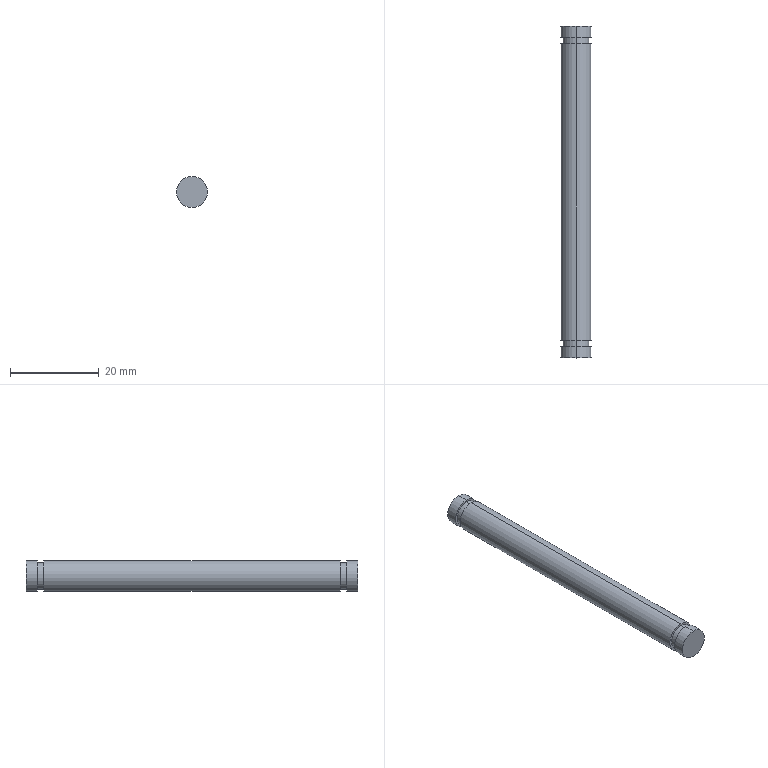Part | SolidWorks | features BaseBody 1 | 1 solid | 16 faces | box 7 x 75 x 7 mm | volume 2856 mm3 | cylinder 10 | plane 6 | commonest cylinder face diameters 7 x6 6 x4
STEP:
#1=CARTESIAN_POINT('',(896.946,-3867.373,951.471));
#2=VERTEX_POINT('',#1);
#3=CARTESIAN_POINT('',(896.946,-3867.373,958.471));
#4=VERTEX_POINT('',#3);
#5=CARTESIAN_POINT('',(896.946,-3867.373,954.971));
#6=DIRECTION('',(0.,-1.,0.));
#7=DIRECTION('',(0.,0.,-1.));
#8=AXIS2_PLACEMENT_3D('',#5,#6,#7);
#9=CIRCLE('',#8,3.5);
#10=EDGE_CURVE('',#2,#4,#9,.T.);
#11=ORIENTED_EDGE('',*,*,#10,.T.);
#12=CARTESIAN_POINT('',(896.946,-3934.373,958.471));
#13=VERTEX_POINT('',#12);
#14=CARTESIAN_POINT('',(896.946,-3903.373,958.471));
#15=DIRECTION('',(0.,-1.,0.));
#16=VECTOR('',#15,1000.);
#17=LINE('',#14,#16);
#18=EDGE_CURVE('',#4,#13,#17,.T.);
#19=ORIENTED_EDGE('',*,*,#18,.T.);
#20=CARTESIAN_POINT('',(896.946,-3934.373,951.471));
#21=VERTEX_POINT('',#20);
#22=CARTESIAN_POINT('',(896.946,-3934.373,954.971));
#23=DIRECTION('',(0.,1.,0.));
#24=DIRECTION('',(0.,0.,-1.));
#25=AXIS2_PLACEMENT_3D('',#22,#23,#24);
#26=CIRCLE('',#25,3.5);
#27=EDGE_CURVE('',#13,#21,#26,.T.);
#28=ORIENTED_EDGE('',*,*,#27,.T.);
#29=CARTESIAN_POINT('',(896.946,-3903.373,951.471));
#30=DIRECTION('',(0.,-1.,0.));
#31=VECTOR('',#30,1000.);
#32=LINE('',#29,#31);
#33=EDGE_CURVE('',#2,#21,#32,.T.);
#34=ORIENTED_EDGE('',*,*,#33,.F.);
#35=EDGE_LOOP('',(#11,#19,#28,#34));
#36=FACE_OUTER_BOUND('',#35,.T.);
#37=CARTESIAN_POINT('',(896.946,-3903.373,954.971));
#38=DIRECTION('',(0.,-1.,0.));
#39=DIRECTION('',(0.,0.,-1.));
#40=AXIS2_PLACEMENT_3D('',#37,#38,#39);
#41=CYLINDRICAL_SURFACE('',#40,3.5);
#42=ADVANCED_FACE('',(#36),#41,.T.);
#43=CARTESIAN_POINT('',(896.946,-3934.373,951.971));
#44=VERTEX_POINT('',#43);
#45=CARTESIAN_POINT('',(896.946,-3934.373,957.971));
#46=VERTEX_POINT('',#45);
#47=CARTESIAN_POINT('',(896.946,-3934.373,954.971));
#48=DIRECTION('',(0.,-1.,0.));
#49=DIRECTION('',(0.,0.,-1.));
#50=AXIS2_PLACEMENT_3D('',#47,#48,#49);
#51=CIRCLE('',#50,3.);
#52=EDGE_CURVE('',#44,#46,#51,.T.);
#53=ORIENTED_EDGE('',*,*,#52,.T.);
#54=CARTESIAN_POINT('',(896.946,-3935.873,957.971));
#55=VERTEX_POINT('',#54);
#56=CARTESIAN_POINT('',(896.946,-3938.667,957.971));
#57=DIRECTION('',(0.,-1.,0.));
#58=VECTOR('',#57,1000.);
#59=LINE('',#56,#58);
#60=EDGE_CURVE('',#46,#55,#59,.T.);
#61=ORIENTED_EDGE('',*,*,#60,.T.);
#62=CARTESIAN_POINT('',(896.946,-3935.873,951.971));
#63=VERTEX_POINT('',#62);
#64=CARTESIAN_POINT('',(896.946,-3935.873,954.971));
#65=DIRECTION('',(0.,1.,0.));
#66=DIRECTION('',(0.,0.,-1.));
#67=AXIS2_PLACEMENT_3D('',#64,#65,#66);
#68=CIRCLE('',#67,3.);
#69=EDGE_CURVE('',#55,#63,#68,.T.);
#70=ORIENTED_EDGE('',*,*,#69,.T.);
#71=CARTESIAN_POINT('',(896.946,-3938.667,951.971));
#72=DIRECTION('',(0.,-1.,0.));
#73=VECTOR('',#72,1000.);
#74=LINE('',#71,#73);
#75=EDGE_CURVE('',#44,#63,#74,.T.);
#76=ORIENTED_EDGE('',*,*,#75,.F.);
#77=EDGE_LOOP('',(#53,#61,#70,#76));
#78=FACE_OUTER_BOUND('',#77,.T.);
#79=CARTESIAN_POINT('',(896.946,-3938.667,954.971));
#80=DIRECTION('',(0.,-1.,0.));
#81=DIRECTION('',(0.,0.,-1.));
#82=AXIS2_PLACEMENT_3D('',#79,#80,#81);
#83=CYLINDRICAL_SURFACE('',#82,3.);
#84=ADVANCED_FACE('',(#78),#83,.T.);
#85=CARTESIAN_POINT('',(896.946,-3865.873,951.971));
#86=VERTEX_POINT('',#85);
#87=CARTESIAN_POINT('',(896.946,-3865.873,957.971));
#88=VERTEX_POINT('',#87);
#89=CARTESIAN_POINT('',(896.946,-3865.873,954.971));
#90=DIRECTION('',(0.,-1.,0.));
#91=DIRECTION('',(0.,0.,-1.));
#92=AXIS2_PLACEMENT_3D('',#89,#90,#91);
#93=CIRCLE('',#92,3.);
#94=EDGE_CURVE('',#86,#88,#93,.T.);
#95=ORIENTED_EDGE('',*,*,#94,.T.);
#96=CARTESIAN_POINT('',(896.946,-3867.373,957.971));
#97=VERTEX_POINT('',#96);
#98=CARTESIAN_POINT('',(896.946,-3870.167,957.971));
#99=DIRECTION('',(0.,-1.,0.));
#100=VECTOR('',#99,1000.);
#101=LINE('',#98,#100);
#102=EDGE_CURVE('',#88,#97,#101,.T.);
#103=ORIENTED_EDGE('',*,*,#102,.T.);
#104=CARTESIAN_POINT('',(896.946,-3867.373,951.971));
#105=VERTEX_POINT('',#104);
#106=CARTESIAN_POINT('',(896.946,-3867.373,954.971));
#107=DIRECTION('',(0.,1.,0.));
#108=DIRECTION('',(0.,0.,-1.));
#109=AXIS2_PLACEMENT_3D('',#106,#107,#108);
#110=CIRCLE('',#109,3.);
#111=EDGE_CURVE('',#97,#105,#110,.T.);
#112=ORIENTED_EDGE('',*,*,#111,.T.);
#113=CARTESIAN_POINT('',(896.946,-3870.167,951.971));
#114=DIRECTION('',(0.,-1.,0.));
#115=VECTOR('',#114,1000.);
#116=LINE('',#113,#115);
#117=EDGE_CURVE('',#86,#105,#116,.T.);
#118=ORIENTED_EDGE('',*,*,#117,.F.);
#119=EDGE_LOOP('',(#95,#103,#112,#118));
#120=FACE_OUTER_BOUND('',#119,.T.);
#121=CARTESIAN_POINT('',(896.946,-3870.167,954.971));
#122=DIRECTION('',(0.,-1.,0.));
#123=DIRECTION('',(0.,0.,-1.));
#124=AXIS2_PLACEMENT_3D('',#121,#122,#123);
#125=CYLINDRICAL_SURFACE('',#124,3.);
#126=ADVANCED_FACE('',(#120),#125,.T.);
#127=CARTESIAN_POINT('',(896.946,-3935.873,951.471));
#128=VERTEX_POINT('',#127);
#129=CARTESIAN_POINT('',(896.946,-3935.873,958.471));
#130=VERTEX_POINT('',#129);
#131=CARTESIAN_POINT('',(896.946,-3935.873,954.971));
#132=DIRECTION('',(0.,-1.,0.));
#133=DIRECTION('',(0.,0.,-1.));
#134=AXIS2_PLACEMENT_3D('',#131,#132,#133);
#135=CIRCLE('',#134,3.5);
#136=EDGE_CURVE('',#128,#130,#135,.T.);
#137=ORIENTED_EDGE('',*,*,#136,.T.);
#138=CARTESIAN_POINT('',(896.946,-3938.373,958.471));
#139=VERTEX_POINT('',#138);
#140=CARTESIAN_POINT('',(896.946,-3903.373,958.471));
#141=DIRECTION('',(0.,-1.,0.));
#142=VECTOR('',#141,1000.);
#143=LINE('',#140,#142);
#144=EDGE_CURVE('',#130,#139,#143,.T.);
#145=ORIENTED_EDGE('',*,*,#144,.T.);
#146=CARTESIAN_POINT('',(896.946,-3938.373,951.471));
#147=VERTEX_POINT('',#146);
#148=CARTESIAN_POINT('',(896.946,-3938.373,954.971));
#149=DIRECTION('',(0.,1.,0.));
#150=DIRECTION('',(0.,0.,-1.));
#151=AXIS2_PLACEMENT_3D('',#148,#149,#150);
#152=CIRCLE('',#151,3.5);
#153=EDGE_CURVE('',#139,#147,#152,.T.);
#154=ORIENTED_EDGE('',*,*,#153,.T.);
#155=CARTESIAN_POINT('',(896.946,-3903.373,951.471));
#156=DIRECTION('',(0.,-1.,0.));
#157=VECTOR('',#156,1000.);
#158=LINE('',#155,#157);
#159=EDGE_CURVE('',#128,#147,#158,.T.);
#160=ORIENTED_EDGE('',*,*,#159,.F.);
#161=EDGE_LOOP('',(#137,#145,#154,#160));
#162=FACE_OUTER_BOUND('',#161,.T.);
#163=CARTESIAN_POINT('',(896.946,-3903.373,954.971));
#164=DIRECTION('',(0.,-1.,0.));
#165=DIRECTION('',(0.,0.,-1.));
#166=AXIS2_PLACEMENT_3D('',#163,#164,#165);
#167=CYLINDRICAL_SURFACE('',#166,3.5);
#168=ADVANCED_FACE('',(#162),#167,.T.);
#169=CARTESIAN_POINT('',(896.946,-3863.373,951.471));
#170=VERTEX_POINT('',#169);
#171=CARTESIAN_POINT('',(896.946,-3863.373,958.471));
#172=VERTEX_POINT('',#171);
#173=CARTESIAN_POINT('',(896.946,-3863.373,954.971));
#174=DIRECTION('',(0.,-1.,0.));
#175=DIRECTION('',(0.,0.,-1.));
#176=AXIS2_PLACEMENT_3D('',#173,#174,#175);
#177=CIRCLE('',#176,3.5);
#178=EDGE_CURVE('',#170,#172,#177,.T.);
#179=ORIENTED_EDGE('',*,*,#178,.T.);
#180=CARTESIAN_POINT('',(896.946,-3865.873,958.471));
#181=VERTEX_POINT('',#180);
#182=CARTESIAN_POINT('',(896.946,-3903.373,958.471));
#183=DIRECTION('',(0.,-1.,0.));
#184=VECTOR('',#183,1000.);
#185=LINE('',#182,#184);
#186=EDGE_CURVE('',#172,#181,#185,.T.);
#187=ORIENTED_EDGE('',*,*,#186,.T.);
#188=CARTESIAN_POINT('',(896.946,-3865.873,951.471));
#189=VERTEX_POINT('',#188);
#190=CARTESIAN_POINT('',(896.946,-3865.873,954.971));
#191=DIRECTION('',(0.,1.,0.));
#192=DIRECTION('',(0.,0.,-1.));
#193=AXIS2_PLACEMENT_3D('',#190,#191,#192);
#194=CIRCLE('',#193,3.5);
#195=EDGE_CURVE('',#181,#189,#194,.T.);
#196=ORIENTED_EDGE('',*,*,#195,.T.);
#197=CARTESIAN_POINT('',(896.946,-3903.373,951.471));
#198=DIRECTION('',(0.,-1.,0.));
#199=VECTOR('',#198,1000.);
#200=LINE('',#197,#199);
#201=EDGE_CURVE('',#170,#189,#200,.T.);
#202=ORIENTED_EDGE('',*,*,#201,.F.);
#203=EDGE_LOOP('',(#179,#187,#196,#202));
#204=FACE_OUTER_BOUND('',#203,.T.);
#205=CARTESIAN_POINT('',(896.946,-3903.373,954.971));
#206=DIRECTION('',(0.,-1.,0.));
#207=DIRECTION('',(0.,0.,-1.));
#208=AXIS2_PLACEMENT_3D('',#205,#206,#207);
#209=CYLINDRICAL_SURFACE('',#208,3.5);
#210=ADVANCED_FACE('',(#204),#209,.T.);
#211=ORIENTED_EDGE('',*,*,#18,.F.);
#212=CARTESIAN_POINT('',(896.946,-3867.373,954.971));
#213=DIRECTION('',(0.,-1.,0.));
#214=DIRECTION('',(0.,0.,-1.));
#215=AXIS2_PLACEMENT_3D('',#212,#213,#214);
#216=CIRCLE('',#215,3.5);
#217=EDGE_CURVE('',#4,#2,#216,.T.);
#218=ORIENTED_EDGE('',*,*,#217,.T.);
#219=ORIENTED_EDGE('',*,*,#33,.T.);
#220=CARTESIAN_POINT('',(896.946,-3934.373,954.971));
#221=DIRECTION('',(0.,1.,0.));
#222=DIRECTION('',(0.,0.,-1.));
#223=AXIS2_PLACEMENT_3D('',#220,#221,#222);
#224=CIRCLE('',#223,3.5);
#225=EDGE_CURVE('',#21,#13,#224,.T.);
#226=ORIENTED_EDGE('',*,*,#225,.T.);
#227=EDGE_LOOP('',(#211,#218,#219,#226));
#228=FACE_OUTER_BOUND('',#227,.T.);
#229=CARTESIAN_POINT('',(896.946,-3903.373,954.971));
#230=DIRECTION('',(0.,-1.,0.));
#231=DIRECTION('',(0.,0.,-1.));
#232=AXIS2_PLACEMENT_3D('',#229,#230,#231);
#233=CYLINDRICAL_SURFACE('',#232,3.5);
#234=ADVANCED_FACE('',(#228),#233,.T.);
#235=ORIENTED_EDGE('',*,*,#52,.F.);
#236=CARTESIAN_POINT('',(896.946,-3934.373,954.971));
#237=DIRECTION('',(0.,-1.,0.));
#238=DIRECTION('',(0.,0.,-1.));
#239=AXIS2_PLACEMENT_3D('',#236,#237,#238);
#240=CIRCLE('',#239,3.);
#241=EDGE_CURVE('',#46,#44,#240,.T.);
#242=ORIENTED_EDGE('',*,*,#241,.F.);
#243=EDGE_LOOP('',(#235,#242));
#244=FACE_BOUND('',#243,.T.);
#245=ORIENTED_EDGE('',*,*,#225,.F.);
#246=ORIENTED_EDGE('',*,*,#27,.F.);
#247=EDGE_LOOP('',(#245,#246));
#248=FACE_OUTER_BOUND('',#247,.T.);
#249=CARTESIAN_POINT('',(896.946,-3934.373,954.971));
#250=DIRECTION('',(0.,1.,0.));
#251=DIRECTION('',(0.,0.,1.));
#252=AXIS2_PLACEMENT_3D('',#249,#250,#251);
#253=PLANE('',#252);
#254=ADVANCED_FACE('',(#244,#248),#253,.F.);
#255=CARTESIAN_POINT('',(896.946,-3867.373,954.971));
#256=DIRECTION('',(0.,1.,0.));
#257=DIRECTION('',(0.,0.,-1.));
#258=AXIS2_PLACEMENT_3D('',#255,#256,#257);
#259=CIRCLE('',#258,3.);
#260=EDGE_CURVE('',#105,#97,#259,.T.);
#261=ORIENTED_EDGE('',*,*,#260,.F.);
#262=ORIENTED_EDGE('',*,*,#111,.F.);
#263=EDGE_LOOP('',(#261,#262));
#264=FACE_BOUND('',#263,.T.);
#265=ORIENTED_EDGE('',*,*,#10,.F.);
#266=ORIENTED_EDGE('',*,*,#217,.F.);
#267=EDGE_LOOP('',(#265,#266));
#268=FACE_OUTER_BOUND('',#267,.T.);
#269=CARTESIAN_POINT('',(896.946,-3867.373,954.971));
#270=DIRECTION('',(0.,-1.,0.));
#271=DIRECTION('',(0.,0.,-1.));
#272=AXIS2_PLACEMENT_3D('',#269,#270,#271);
#273=PLANE('',#272);
#274=ADVANCED_FACE('',(#264,#268),#273,.F.);
#275=ORIENTED_EDGE('',*,*,#60,.F.);
#276=ORIENTED_EDGE('',*,*,#241,.T.);
#277=ORIENTED_EDGE('',*,*,#75,.T.);
#278=CARTESIAN_POINT('',(896.946,-3935.873,954.971));
#279=DIRECTION('',(0.,1.,0.));
#280=DIRECTION('',(0.,0.,-1.));
#281=AXIS2_PLACEMENT_3D('',#278,#279,#280);
#282=CIRCLE('',#281,3.);
#283=EDGE_CURVE('',#63,#55,#282,.T.);
#284=ORIENTED_EDGE('',*,*,#283,.T.);
#285=EDGE_LOOP('',(#275,#276,#277,#284));
#286=FACE_OUTER_BOUND('',#285,.T.);
#287=CARTESIAN_POINT('',(896.946,-3938.667,954.971));
#288=DIRECTION('',(0.,-1.,0.));
#289=DIRECTION('',(0.,0.,-1.));
#290=AXIS2_PLACEMENT_3D('',#287,#288,#289);
#291=CYLINDRICAL_SURFACE('',#290,3.);
#292=ADVANCED_FACE('',(#286),#291,.T.);
#293=ORIENTED_EDGE('',*,*,#102,.F.);
#294=CARTESIAN_POINT('',(896.946,-3865.873,954.971));
#295=DIRECTION('',(0.,-1.,0.));
#296=DIRECTION('',(0.,0.,-1.));
#297=AXIS2_PLACEMENT_3D('',#294,#295,#296);
#298=CIRCLE('',#297,3.);
#299=EDGE_CURVE('',#88,#86,#298,.T.);
#300=ORIENTED_EDGE('',*,*,#299,.T.);
#301=ORIENTED_EDGE('',*,*,#117,.T.);
#302=ORIENTED_EDGE('',*,*,#260,.T.);
#303=EDGE_LOOP('',(#293,#300,#301,#302));
#304=FACE_OUTER_BOUND('',#303,.T.);
#305=CARTESIAN_POINT('',(896.946,-3870.167,954.971));
#306=DIRECTION('',(0.,-1.,0.));
#307=DIRECTION('',(0.,0.,-1.));
#308=AXIS2_PLACEMENT_3D('',#305,#306,#307);
#309=CYLINDRICAL_SURFACE('',#308,3.);
#310=ADVANCED_FACE('',(#304),#309,.T.);
#311=ORIENTED_EDGE('',*,*,#283,.F.);
#312=ORIENTED_EDGE('',*,*,#69,.F.);
#313=EDGE_LOOP('',(#311,#312));
#314=FACE_BOUND('',#313,.T.);
#315=ORIENTED_EDGE('',*,*,#136,.F.);
#316=CARTESIAN_POINT('',(896.946,-3935.873,954.971));
#317=DIRECTION('',(0.,-1.,0.));
#318=DIRECTION('',(0.,0.,-1.));
#319=AXIS2_PLACEMENT_3D('',#316,#317,#318);
#320=CIRCLE('',#319,3.5);
#321=EDGE_CURVE('',#130,#128,#320,.T.);
#322=ORIENTED_EDGE('',*,*,#321,.F.);
#323=EDGE_LOOP('',(#315,#322));
#324=FACE_OUTER_BOUND('',#323,.T.);
#325=CARTESIAN_POINT('',(896.946,-3935.873,954.971));
#326=DIRECTION('',(0.,-1.,0.));
#327=DIRECTION('',(0.,0.,-1.));
#328=AXIS2_PLACEMENT_3D('',#325,#326,#327);
#329=PLANE('',#328);
#330=ADVANCED_FACE('',(#314,#324),#329,.F.);
#331=ORIENTED_EDGE('',*,*,#94,.F.);
#332=ORIENTED_EDGE('',*,*,#299,.F.);
#333=EDGE_LOOP('',(#331,#332));
#334=FACE_BOUND('',#333,.T.);
#335=CARTESIAN_POINT('',(896.946,-3865.873,954.971));
#336=DIRECTION('',(0.,1.,0.));
#337=DIRECTION('',(0.,0.,-1.));
#338=AXIS2_PLACEMENT_3D('',#335,#336,#337);
#339=CIRCLE('',#338,3.5);
#340=EDGE_CURVE('',#189,#181,#339,.T.);
#341=ORIENTED_EDGE('',*,*,#340,.F.);
#342=ORIENTED_EDGE('',*,*,#195,.F.);
#343=EDGE_LOOP('',(#341,#342));
#344=FACE_OUTER_BOUND('',#343,.T.);
#345=CARTESIAN_POINT('',(896.946,-3865.873,954.971));
#346=DIRECTION('',(0.,1.,0.));
#347=DIRECTION('',(0.,0.,1.));
#348=AXIS2_PLACEMENT_3D('',#345,#346,#347);
#349=PLANE('',#348);
#350=ADVANCED_FACE('',(#334,#344),#349,.F.);
#351=ORIENTED_EDGE('',*,*,#144,.F.);
#352=ORIENTED_EDGE('',*,*,#321,.T.);
#353=ORIENTED_EDGE('',*,*,#159,.T.);
#354=CARTESIAN_POINT('',(896.946,-3938.373,954.971));
#355=DIRECTION('',(0.,1.,0.));
#356=DIRECTION('',(0.,0.,-1.));
#357=AXIS2_PLACEMENT_3D('',#354,#355,#356);
#358=CIRCLE('',#357,3.5);
#359=EDGE_CURVE('',#147,#139,#358,.T.);
#360=ORIENTED_EDGE('',*,*,#359,.T.);
#361=EDGE_LOOP('',(#351,#352,#353,#360));
#362=FACE_OUTER_BOUND('',#361,.T.);
#363=CARTESIAN_POINT('',(896.946,-3903.373,954.971));
#364=DIRECTION('',(0.,-1.,0.));
#365=DIRECTION('',(0.,0.,-1.));
#366=AXIS2_PLACEMENT_3D('',#363,#364,#365);
#367=CYLINDRICAL_SURFACE('',#366,3.5);
#368=ADVANCED_FACE('',(#362),#367,.T.);
#369=ORIENTED_EDGE('',*,*,#186,.F.);
#370=CARTESIAN_POINT('',(896.946,-3863.373,954.971));
#371=DIRECTION('',(0.,-1.,0.));
#372=DIRECTION('',(0.,0.,-1.));
#373=AXIS2_PLACEMENT_3D('',#370,#371,#372);
#374=CIRCLE('',#373,3.5);
#375=EDGE_CURVE('',#172,#170,#374,.T.);
#376=ORIENTED_EDGE('',*,*,#375,.T.);
#377=ORIENTED_EDGE('',*,*,#201,.T.);
#378=ORIENTED_EDGE('',*,*,#340,.T.);
#379=EDGE_LOOP('',(#369,#376,#377,#378));
#380=FACE_OUTER_BOUND('',#379,.T.);
#381=CARTESIAN_POINT('',(896.946,-3903.373,954.971));
#382=DIRECTION('',(0.,-1.,0.));
#383=DIRECTION('',(0.,0.,-1.));
#384=AXIS2_PLACEMENT_3D('',#381,#382,#383);
#385=CYLINDRICAL_SURFACE('',#384,3.5);
#386=ADVANCED_FACE('',(#380),#385,.T.);
#387=ORIENTED_EDGE('',*,*,#359,.F.);
#388=ORIENTED_EDGE('',*,*,#153,.F.);
#389=EDGE_LOOP('',(#387,#388));
#390=FACE_OUTER_BOUND('',#389,.T.);
#391=CARTESIAN_POINT('',(896.946,-3938.373,954.971));
#392=DIRECTION('',(0.,-1.,0.));
#393=DIRECTION('',(0.,0.,-1.));
#394=AXIS2_PLACEMENT_3D('',#391,#392,#393);
#395=PLANE('',#394);
#396=ADVANCED_FACE('',(#390),#395,.T.);
#397=ORIENTED_EDGE('',*,*,#178,.F.);
#398=ORIENTED_EDGE('',*,*,#375,.F.);
#399=EDGE_LOOP('',(#397,#398));
#400=FACE_OUTER_BOUND('',#399,.T.);
#401=CARTESIAN_POINT('',(896.946,-3863.373,954.971));
#402=DIRECTION('',(0.,1.,0.));
#403=DIRECTION('',(0.,0.,1.));
#404=AXIS2_PLACEMENT_3D('',#401,#402,#403);
#405=PLANE('',#404);
#406=ADVANCED_FACE('',(#400),#405,.T.);
#407=CLOSED_SHELL('',(#42,#84,#126,#168,#210,#234,#254,#274,#292,#310,#330,#350,#368,#386,#396,#406));
#408=MANIFOLD_SOLID_BREP('',#407);
#409=CARTESIAN_POINT('',(0.,0.,0.));
#410=DIRECTION('',(0.,0.,1.));
#411=DIRECTION('',(1.,0.,0.));
#412=AXIS2_PLACEMENT_3D('',#409,#410,#411);
#413=(LENGTH_UNIT()NAMED_UNIT(*)SI_UNIT(.MILLI.,.METRE.));
#414=UNCERTAINTY_MEASURE_WITH_UNIT(LENGTH_MEASURE(0.00001),#413,'','');
#415=(NAMED_UNIT(*)PLANE_ANGLE_UNIT()SI_UNIT($,.RADIAN.));
#416=(NAMED_UNIT(*)SI_UNIT($,.STERADIAN.)SOLID_ANGLE_UNIT());
#417=(GEOMETRIC_REPRESENTATION_CONTEXT(3)GLOBAL_UNCERTAINTY_ASSIGNED_CONTEXT((#414))GLOBAL_UNIT_ASSIGNED_CONTEXT((#413,#415,#416))REPRESENTATION_CONTEXT('',''));
#418=ADVANCED_BREP_SHAPE_REPRESENTATION('',(#408,#412),#417);